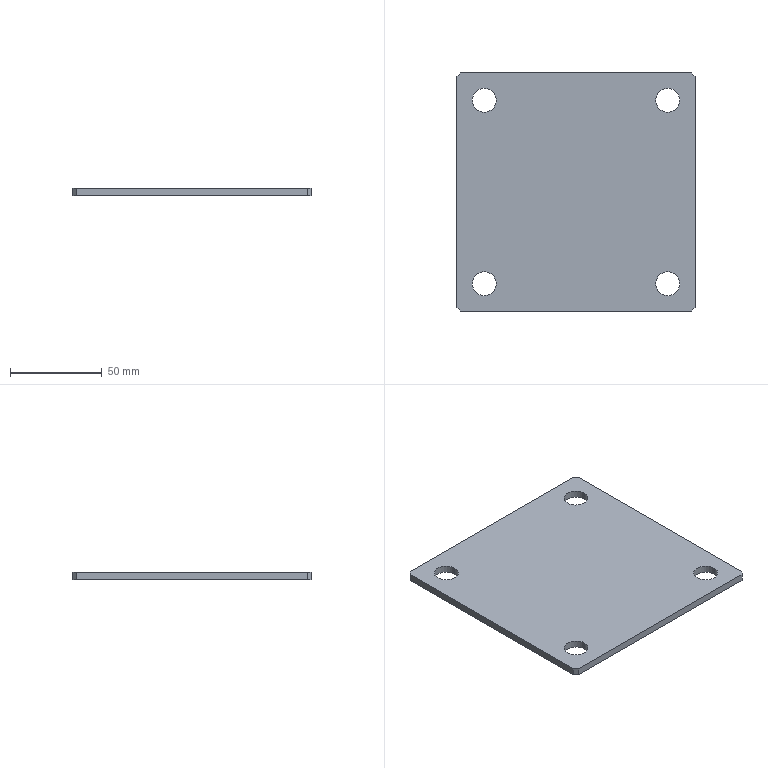Part | SolidWorks | features Chamfer 1, Extrusion 1, HoleWzd 1 | 1 solid | 18 faces | box 130 x 130 x 4 mm | volume 65444 mm3 | plane 10 | cylinder 8 | commonest cylinder face diameters 13 x8
STEP:
#1=CARTESIAN_POINT('',(-8.5,50.,4.));
#2=VERTEX_POINT('',#1);
#3=CARTESIAN_POINT('',(-21.5,50.,4.));
#4=VERTEX_POINT('',#3);
#5=CARTESIAN_POINT('',(-15.,50.,4.));
#6=DIRECTION('',(0.,0.,-1.));
#7=DIRECTION('',(-1.,0.,0.));
#8=AXIS2_PLACEMENT_3D('',#5,#6,#7);
#9=CIRCLE('',#8,6.5);
#10=EDGE_CURVE('',#2,#4,#9,.T.);
#11=ORIENTED_EDGE('',*,*,#10,.F.);
#12=CARTESIAN_POINT('',(-8.5,50.,0.));
#13=VERTEX_POINT('',#12);
#14=CARTESIAN_POINT('',(-8.5,50.,0.));
#15=DIRECTION('',(0.,0.,-1.));
#16=VECTOR('',#15,1000.);
#17=LINE('',#14,#16);
#18=EDGE_CURVE('',#2,#13,#17,.T.);
#19=ORIENTED_EDGE('',*,*,#18,.T.);
#20=CARTESIAN_POINT('',(-21.5,50.,0.));
#21=VERTEX_POINT('',#20);
#22=CARTESIAN_POINT('',(-15.,50.,0.));
#23=DIRECTION('',(0.,0.,-1.));
#24=DIRECTION('',(-1.,0.,0.));
#25=AXIS2_PLACEMENT_3D('',#22,#23,#24);
#26=CIRCLE('',#25,6.5);
#27=EDGE_CURVE('',#13,#21,#26,.T.);
#28=ORIENTED_EDGE('',*,*,#27,.T.);
#29=CARTESIAN_POINT('',(-21.5,50.,0.));
#30=DIRECTION('',(0.,0.,-1.));
#31=VECTOR('',#30,1000.);
#32=LINE('',#29,#31);
#33=EDGE_CURVE('',#4,#21,#32,.T.);
#34=ORIENTED_EDGE('',*,*,#33,.F.);
#35=EDGE_LOOP('',(#11,#19,#28,#34));
#36=FACE_OUTER_BOUND('',#35,.T.);
#37=CARTESIAN_POINT('',(-15.,50.,0.));
#38=DIRECTION('',(0.,0.,-1.));
#39=DIRECTION('',(-1.,0.,0.));
#40=AXIS2_PLACEMENT_3D('',#37,#38,#39);
#41=CYLINDRICAL_SURFACE('',#40,6.5);
#42=ADVANCED_FACE('',(#36),#41,.F.);
#43=CARTESIAN_POINT('',(-108.5,-50.,4.));
#44=VERTEX_POINT('',#43);
#45=CARTESIAN_POINT('',(-121.5,-50.,4.));
#46=VERTEX_POINT('',#45);
#47=CARTESIAN_POINT('',(-115.,-50.,4.));
#48=DIRECTION('',(0.,0.,-1.));
#49=DIRECTION('',(-1.,0.,0.));
#50=AXIS2_PLACEMENT_3D('',#47,#48,#49);
#51=CIRCLE('',#50,6.5);
#52=EDGE_CURVE('',#44,#46,#51,.T.);
#53=ORIENTED_EDGE('',*,*,#52,.F.);
#54=CARTESIAN_POINT('',(-108.5,-50.,0.));
#55=VERTEX_POINT('',#54);
#56=CARTESIAN_POINT('',(-108.5,-50.,0.));
#57=DIRECTION('',(0.,0.,-1.));
#58=VECTOR('',#57,1000.);
#59=LINE('',#56,#58);
#60=EDGE_CURVE('',#44,#55,#59,.T.);
#61=ORIENTED_EDGE('',*,*,#60,.T.);
#62=CARTESIAN_POINT('',(-121.5,-50.,0.));
#63=VERTEX_POINT('',#62);
#64=CARTESIAN_POINT('',(-115.,-50.,0.));
#65=DIRECTION('',(0.,0.,-1.));
#66=DIRECTION('',(-1.,0.,0.));
#67=AXIS2_PLACEMENT_3D('',#64,#65,#66);
#68=CIRCLE('',#67,6.5);
#69=EDGE_CURVE('',#55,#63,#68,.T.);
#70=ORIENTED_EDGE('',*,*,#69,.T.);
#71=CARTESIAN_POINT('',(-121.5,-50.,0.));
#72=DIRECTION('',(0.,0.,-1.));
#73=VECTOR('',#72,1000.);
#74=LINE('',#71,#73);
#75=EDGE_CURVE('',#46,#63,#74,.T.);
#76=ORIENTED_EDGE('',*,*,#75,.F.);
#77=EDGE_LOOP('',(#53,#61,#70,#76));
#78=FACE_OUTER_BOUND('',#77,.T.);
#79=CARTESIAN_POINT('',(-115.,-50.,0.));
#80=DIRECTION('',(0.,0.,-1.));
#81=DIRECTION('',(-1.,0.,0.));
#82=AXIS2_PLACEMENT_3D('',#79,#80,#81);
#83=CYLINDRICAL_SURFACE('',#82,6.5);
#84=ADVANCED_FACE('',(#78),#83,.F.);
#85=CARTESIAN_POINT('',(-108.5,50.,4.));
#86=VERTEX_POINT('',#85);
#87=CARTESIAN_POINT('',(-121.5,50.,4.));
#88=VERTEX_POINT('',#87);
#89=CARTESIAN_POINT('',(-115.,50.,4.));
#90=DIRECTION('',(0.,0.,-1.));
#91=DIRECTION('',(-1.,0.,0.));
#92=AXIS2_PLACEMENT_3D('',#89,#90,#91);
#93=CIRCLE('',#92,6.5);
#94=EDGE_CURVE('',#86,#88,#93,.T.);
#95=ORIENTED_EDGE('',*,*,#94,.F.);
#96=CARTESIAN_POINT('',(-108.5,50.,0.));
#97=VERTEX_POINT('',#96);
#98=CARTESIAN_POINT('',(-108.5,50.,0.));
#99=DIRECTION('',(0.,0.,-1.));
#100=VECTOR('',#99,1000.);
#101=LINE('',#98,#100);
#102=EDGE_CURVE('',#86,#97,#101,.T.);
#103=ORIENTED_EDGE('',*,*,#102,.T.);
#104=CARTESIAN_POINT('',(-121.5,50.,0.));
#105=VERTEX_POINT('',#104);
#106=CARTESIAN_POINT('',(-115.,50.,0.));
#107=DIRECTION('',(0.,0.,-1.));
#108=DIRECTION('',(-1.,0.,0.));
#109=AXIS2_PLACEMENT_3D('',#106,#107,#108);
#110=CIRCLE('',#109,6.5);
#111=EDGE_CURVE('',#97,#105,#110,.T.);
#112=ORIENTED_EDGE('',*,*,#111,.T.);
#113=CARTESIAN_POINT('',(-121.5,50.,0.));
#114=DIRECTION('',(0.,0.,-1.));
#115=VECTOR('',#114,1000.);
#116=LINE('',#113,#115);
#117=EDGE_CURVE('',#88,#105,#116,.T.);
#118=ORIENTED_EDGE('',*,*,#117,.F.);
#119=EDGE_LOOP('',(#95,#103,#112,#118));
#120=FACE_OUTER_BOUND('',#119,.T.);
#121=CARTESIAN_POINT('',(-115.,50.,0.));
#122=DIRECTION('',(0.,0.,-1.));
#123=DIRECTION('',(-1.,0.,0.));
#124=AXIS2_PLACEMENT_3D('',#121,#122,#123);
#125=CYLINDRICAL_SURFACE('',#124,6.5);
#126=ADVANCED_FACE('',(#120),#125,.F.);
#127=CARTESIAN_POINT('',(-8.5,-50.,4.));
#128=VERTEX_POINT('',#127);
#129=CARTESIAN_POINT('',(-21.5,-50.,4.));
#130=VERTEX_POINT('',#129);
#131=CARTESIAN_POINT('',(-15.,-50.,4.));
#132=DIRECTION('',(0.,0.,-1.));
#133=DIRECTION('',(-1.,0.,0.));
#134=AXIS2_PLACEMENT_3D('',#131,#132,#133);
#135=CIRCLE('',#134,6.5);
#136=EDGE_CURVE('',#128,#130,#135,.T.);
#137=ORIENTED_EDGE('',*,*,#136,.F.);
#138=CARTESIAN_POINT('',(-8.5,-50.,0.));
#139=VERTEX_POINT('',#138);
#140=CARTESIAN_POINT('',(-8.5,-50.,0.));
#141=DIRECTION('',(0.,0.,-1.));
#142=VECTOR('',#141,1000.);
#143=LINE('',#140,#142);
#144=EDGE_CURVE('',#128,#139,#143,.T.);
#145=ORIENTED_EDGE('',*,*,#144,.T.);
#146=CARTESIAN_POINT('',(-21.5,-50.,0.));
#147=VERTEX_POINT('',#146);
#148=CARTESIAN_POINT('',(-15.,-50.,0.));
#149=DIRECTION('',(0.,0.,-1.));
#150=DIRECTION('',(-1.,0.,0.));
#151=AXIS2_PLACEMENT_3D('',#148,#149,#150);
#152=CIRCLE('',#151,6.5);
#153=EDGE_CURVE('',#139,#147,#152,.T.);
#154=ORIENTED_EDGE('',*,*,#153,.T.);
#155=CARTESIAN_POINT('',(-21.5,-50.,0.));
#156=DIRECTION('',(0.,0.,-1.));
#157=VECTOR('',#156,1000.);
#158=LINE('',#155,#157);
#159=EDGE_CURVE('',#130,#147,#158,.T.);
#160=ORIENTED_EDGE('',*,*,#159,.F.);
#161=EDGE_LOOP('',(#137,#145,#154,#160));
#162=FACE_OUTER_BOUND('',#161,.T.);
#163=CARTESIAN_POINT('',(-15.,-50.,0.));
#164=DIRECTION('',(0.,0.,-1.));
#165=DIRECTION('',(-1.,0.,0.));
#166=AXIS2_PLACEMENT_3D('',#163,#164,#165);
#167=CYLINDRICAL_SURFACE('',#166,6.5);
#168=ADVANCED_FACE('',(#162),#167,.F.);
#169=CARTESIAN_POINT('',(0.,-63.,4.));
#170=VERTEX_POINT('',#169);
#171=CARTESIAN_POINT('',(0.,63.,4.));
#172=VERTEX_POINT('',#171);
#173=CARTESIAN_POINT('',(0.,65.,4.));
#174=DIRECTION('',(0.,1.,0.));
#175=VECTOR('',#174,1000.);
#176=LINE('',#173,#175);
#177=EDGE_CURVE('',#170,#172,#176,.T.);
#178=ORIENTED_EDGE('',*,*,#177,.F.);
#179=CARTESIAN_POINT('',(0.,-63.,0.));
#180=VERTEX_POINT('',#179);
#181=CARTESIAN_POINT('',(0.,-63.,4.));
#182=DIRECTION('',(0.,0.,-1.));
#183=VECTOR('',#182,1000.);
#184=LINE('',#181,#183);
#185=EDGE_CURVE('',#170,#180,#184,.T.);
#186=ORIENTED_EDGE('',*,*,#185,.T.);
#187=CARTESIAN_POINT('',(0.,63.,0.));
#188=VERTEX_POINT('',#187);
#189=CARTESIAN_POINT('',(0.,65.,0.));
#190=DIRECTION('',(0.,1.,0.));
#191=VECTOR('',#190,1000.);
#192=LINE('',#189,#191);
#193=EDGE_CURVE('',#180,#188,#192,.T.);
#194=ORIENTED_EDGE('',*,*,#193,.T.);
#195=CARTESIAN_POINT('',(0.,63.,4.));
#196=DIRECTION('',(0.,0.,1.));
#197=VECTOR('',#196,1000.);
#198=LINE('',#195,#197);
#199=EDGE_CURVE('',#188,#172,#198,.T.);
#200=ORIENTED_EDGE('',*,*,#199,.T.);
#201=EDGE_LOOP('',(#178,#186,#194,#200));
#202=FACE_OUTER_BOUND('',#201,.T.);
#203=CARTESIAN_POINT('',(0.,65.,4.));
#204=DIRECTION('',(-1.,0.,0.));
#205=DIRECTION('',(0.,-1.,0.));
#206=AXIS2_PLACEMENT_3D('',#203,#204,#205);
#207=PLANE('',#206);
#208=ADVANCED_FACE('',(#202),#207,.F.);
#209=CARTESIAN_POINT('',(-2.,65.,0.));
#210=VERTEX_POINT('',#209);
#211=CARTESIAN_POINT('',(-128.,65.,0.));
#212=VERTEX_POINT('',#211);
#213=CARTESIAN_POINT('',(0.,65.,0.));
#214=DIRECTION('',(-1.,0.,0.));
#215=VECTOR('',#214,1000.);
#216=LINE('',#213,#215);
#217=EDGE_CURVE('',#210,#212,#216,.T.);
#218=ORIENTED_EDGE('',*,*,#217,.T.);
#219=CARTESIAN_POINT('',(-128.,65.,4.));
#220=VERTEX_POINT('',#219);
#221=CARTESIAN_POINT('',(-128.,65.,4.));
#222=DIRECTION('',(0.,0.,1.));
#223=VECTOR('',#222,1000.);
#224=LINE('',#221,#223);
#225=EDGE_CURVE('',#212,#220,#224,.T.);
#226=ORIENTED_EDGE('',*,*,#225,.T.);
#227=CARTESIAN_POINT('',(-2.,65.,4.));
#228=VERTEX_POINT('',#227);
#229=CARTESIAN_POINT('',(0.,65.,4.));
#230=DIRECTION('',(-1.,0.,0.));
#231=VECTOR('',#230,1000.);
#232=LINE('',#229,#231);
#233=EDGE_CURVE('',#228,#220,#232,.T.);
#234=ORIENTED_EDGE('',*,*,#233,.F.);
#235=CARTESIAN_POINT('',(-2.,65.,4.));
#236=DIRECTION('',(0.,0.,-1.));
#237=VECTOR('',#236,1000.);
#238=LINE('',#235,#237);
#239=EDGE_CURVE('',#228,#210,#238,.T.);
#240=ORIENTED_EDGE('',*,*,#239,.T.);
#241=EDGE_LOOP('',(#218,#226,#234,#240));
#242=FACE_OUTER_BOUND('',#241,.T.);
#243=CARTESIAN_POINT('',(0.,65.,4.));
#244=DIRECTION('',(0.,-1.,0.));
#245=DIRECTION('',(0.,0.,-1.));
#246=AXIS2_PLACEMENT_3D('',#243,#244,#245);
#247=PLANE('',#246);
#248=ADVANCED_FACE('',(#242),#247,.F.);
#249=CARTESIAN_POINT('',(-130.,63.,4.));
#250=VERTEX_POINT('',#249);
#251=CARTESIAN_POINT('',(-130.,-63.,4.));
#252=VERTEX_POINT('',#251);
#253=CARTESIAN_POINT('',(-130.,65.,4.));
#254=DIRECTION('',(0.,-1.,0.));
#255=VECTOR('',#254,1000.);
#256=LINE('',#253,#255);
#257=EDGE_CURVE('',#250,#252,#256,.T.);
#258=ORIENTED_EDGE('',*,*,#257,.F.);
#259=CARTESIAN_POINT('',(-130.,63.,0.));
#260=VERTEX_POINT('',#259);
#261=CARTESIAN_POINT('',(-130.,63.,4.));
#262=DIRECTION('',(0.,0.,-1.));
#263=VECTOR('',#262,1000.);
#264=LINE('',#261,#263);
#265=EDGE_CURVE('',#250,#260,#264,.T.);
#266=ORIENTED_EDGE('',*,*,#265,.T.);
#267=CARTESIAN_POINT('',(-130.,-63.,0.));
#268=VERTEX_POINT('',#267);
#269=CARTESIAN_POINT('',(-130.,65.,0.));
#270=DIRECTION('',(0.,-1.,0.));
#271=VECTOR('',#270,1000.);
#272=LINE('',#269,#271);
#273=EDGE_CURVE('',#260,#268,#272,.T.);
#274=ORIENTED_EDGE('',*,*,#273,.T.);
#275=CARTESIAN_POINT('',(-130.,-63.,4.));
#276=DIRECTION('',(0.,0.,1.));
#277=VECTOR('',#276,1000.);
#278=LINE('',#275,#277);
#279=EDGE_CURVE('',#268,#252,#278,.T.);
#280=ORIENTED_EDGE('',*,*,#279,.T.);
#281=EDGE_LOOP('',(#258,#266,#274,#280));
#282=FACE_OUTER_BOUND('',#281,.T.);
#283=CARTESIAN_POINT('',(-130.,65.,4.));
#284=DIRECTION('',(1.,0.,0.));
#285=DIRECTION('',(0.,1.,0.));
#286=AXIS2_PLACEMENT_3D('',#283,#284,#285);
#287=PLANE('',#286);
#288=ADVANCED_FACE('',(#282),#287,.F.);
#289=CARTESIAN_POINT('',(-128.,-65.,4.));
#290=VERTEX_POINT('',#289);
#291=CARTESIAN_POINT('',(-2.,-65.,4.));
#292=VERTEX_POINT('',#291);
#293=CARTESIAN_POINT('',(0.,-65.,4.));
#294=DIRECTION('',(1.,0.,0.));
#295=VECTOR('',#294,1000.);
#296=LINE('',#293,#295);
#297=EDGE_CURVE('',#290,#292,#296,.T.);
#298=ORIENTED_EDGE('',*,*,#297,.F.);
#299=CARTESIAN_POINT('',(-128.,-65.,0.));
#300=VERTEX_POINT('',#299);
#301=CARTESIAN_POINT('',(-128.,-65.,4.));
#302=DIRECTION('',(0.,0.,-1.));
#303=VECTOR('',#302,1000.);
#304=LINE('',#301,#303);
#305=EDGE_CURVE('',#290,#300,#304,.T.);
#306=ORIENTED_EDGE('',*,*,#305,.T.);
#307=CARTESIAN_POINT('',(-2.,-65.,0.));
#308=VERTEX_POINT('',#307);
#309=CARTESIAN_POINT('',(0.,-65.,0.));
#310=DIRECTION('',(1.,0.,0.));
#311=VECTOR('',#310,1000.);
#312=LINE('',#309,#311);
#313=EDGE_CURVE('',#300,#308,#312,.T.);
#314=ORIENTED_EDGE('',*,*,#313,.T.);
#315=CARTESIAN_POINT('',(-2.,-65.,4.));
#316=DIRECTION('',(0.,0.,1.));
#317=VECTOR('',#316,1000.);
#318=LINE('',#315,#317);
#319=EDGE_CURVE('',#308,#292,#318,.T.);
#320=ORIENTED_EDGE('',*,*,#319,.T.);
#321=EDGE_LOOP('',(#298,#306,#314,#320));
#322=FACE_OUTER_BOUND('',#321,.T.);
#323=CARTESIAN_POINT('',(0.,-65.,4.));
#324=DIRECTION('',(0.,1.,0.));
#325=DIRECTION('',(-1.,0.,0.));
#326=AXIS2_PLACEMENT_3D('',#323,#324,#325);
#327=PLANE('',#326);
#328=ADVANCED_FACE('',(#322),#327,.F.);
#329=CARTESIAN_POINT('',(-15.,50.,4.));
#330=DIRECTION('',(0.,0.,-1.));
#331=DIRECTION('',(-1.,0.,0.));
#332=AXIS2_PLACEMENT_3D('',#329,#330,#331);
#333=CIRCLE('',#332,6.5);
#334=EDGE_CURVE('',#4,#2,#333,.T.);
#335=ORIENTED_EDGE('',*,*,#334,.T.);
#336=ORIENTED_EDGE('',*,*,#10,.T.);
#337=EDGE_LOOP('',(#335,#336));
#338=FACE_BOUND('',#337,.T.);
#339=CARTESIAN_POINT('',(-115.,-50.,4.));
#340=DIRECTION('',(0.,0.,-1.));
#341=DIRECTION('',(-1.,0.,0.));
#342=AXIS2_PLACEMENT_3D('',#339,#340,#341);
#343=CIRCLE('',#342,6.5);
#344=EDGE_CURVE('',#46,#44,#343,.T.);
#345=ORIENTED_EDGE('',*,*,#344,.T.);
#346=ORIENTED_EDGE('',*,*,#52,.T.);
#347=EDGE_LOOP('',(#345,#346));
#348=FACE_BOUND('',#347,.T.);
#349=CARTESIAN_POINT('',(-115.,50.,4.));
#350=DIRECTION('',(0.,0.,-1.));
#351=DIRECTION('',(-1.,0.,0.));
#352=AXIS2_PLACEMENT_3D('',#349,#350,#351);
#353=CIRCLE('',#352,6.5);
#354=EDGE_CURVE('',#88,#86,#353,.T.);
#355=ORIENTED_EDGE('',*,*,#354,.T.);
#356=ORIENTED_EDGE('',*,*,#94,.T.);
#357=EDGE_LOOP('',(#355,#356));
#358=FACE_BOUND('',#357,.T.);
#359=CARTESIAN_POINT('',(-15.,-50.,4.));
#360=DIRECTION('',(0.,0.,-1.));
#361=DIRECTION('',(-1.,0.,0.));
#362=AXIS2_PLACEMENT_3D('',#359,#360,#361);
#363=CIRCLE('',#362,6.5);
#364=EDGE_CURVE('',#130,#128,#363,.T.);
#365=ORIENTED_EDGE('',*,*,#364,.T.);
#366=ORIENTED_EDGE('',*,*,#136,.T.);
#367=EDGE_LOOP('',(#365,#366));
#368=FACE_BOUND('',#367,.T.);
#369=ORIENTED_EDGE('',*,*,#233,.T.);
#370=CARTESIAN_POINT('',(-130.,63.,4.));
#371=DIRECTION('',(-0.7071,-0.7071,0.));
#372=VECTOR('',#371,1000.);
#373=LINE('',#370,#372);
#374=EDGE_CURVE('',#220,#250,#373,.T.);
#375=ORIENTED_EDGE('',*,*,#374,.T.);
#376=ORIENTED_EDGE('',*,*,#257,.T.);
#377=CARTESIAN_POINT('',(-128.,-65.,4.));
#378=DIRECTION('',(0.7071,-0.7071,0.));
#379=VECTOR('',#378,1000.);
#380=LINE('',#377,#379);
#381=EDGE_CURVE('',#252,#290,#380,.T.);
#382=ORIENTED_EDGE('',*,*,#381,.T.);
#383=ORIENTED_EDGE('',*,*,#297,.T.);
#384=CARTESIAN_POINT('',(0.,-63.,4.));
#385=DIRECTION('',(0.7071,0.7071,0.));
#386=VECTOR('',#385,1000.);
#387=LINE('',#384,#386);
#388=EDGE_CURVE('',#292,#170,#387,.T.);
#389=ORIENTED_EDGE('',*,*,#388,.T.);
#390=ORIENTED_EDGE('',*,*,#177,.T.);
#391=CARTESIAN_POINT('',(-2.,65.,4.));
#392=DIRECTION('',(-0.7071,0.7071,0.));
#393=VECTOR('',#392,1000.);
#394=LINE('',#391,#393);
#395=EDGE_CURVE('',#172,#228,#394,.T.);
#396=ORIENTED_EDGE('',*,*,#395,.T.);
#397=EDGE_LOOP('',(#369,#375,#376,#382,#383,#389,#390,#396));
#398=FACE_OUTER_BOUND('',#397,.T.);
#399=CARTESIAN_POINT('',(0.,0.,4.));
#400=DIRECTION('',(0.,0.,-1.));
#401=DIRECTION('',(-1.,0.,0.));
#402=AXIS2_PLACEMENT_3D('',#399,#400,#401);
#403=PLANE('',#402);
#404=ADVANCED_FACE('',(#338,#348,#358,#368,#398),#403,.F.);
#405=CARTESIAN_POINT('',(-15.,50.,0.));
#406=DIRECTION('',(0.,0.,-1.));
#407=DIRECTION('',(-1.,0.,0.));
#408=AXIS2_PLACEMENT_3D('',#405,#406,#407);
#409=CIRCLE('',#408,6.5);
#410=EDGE_CURVE('',#21,#13,#409,.T.);
#411=ORIENTED_EDGE('',*,*,#410,.F.);
#412=ORIENTED_EDGE('',*,*,#27,.F.);
#413=EDGE_LOOP('',(#411,#412));
#414=FACE_BOUND('',#413,.T.);
#415=CARTESIAN_POINT('',(-115.,-50.,0.));
#416=DIRECTION('',(0.,0.,-1.));
#417=DIRECTION('',(-1.,0.,0.));
#418=AXIS2_PLACEMENT_3D('',#415,#416,#417);
#419=CIRCLE('',#418,6.5);
#420=EDGE_CURVE('',#63,#55,#419,.T.);
#421=ORIENTED_EDGE('',*,*,#420,.F.);
#422=ORIENTED_EDGE('',*,*,#69,.F.);
#423=EDGE_LOOP('',(#421,#422));
#424=FACE_BOUND('',#423,.T.);
#425=CARTESIAN_POINT('',(-115.,50.,0.));
#426=DIRECTION('',(0.,0.,-1.));
#427=DIRECTION('',(-1.,0.,0.));
#428=AXIS2_PLACEMENT_3D('',#425,#426,#427);
#429=CIRCLE('',#428,6.5);
#430=EDGE_CURVE('',#105,#97,#429,.T.);
#431=ORIENTED_EDGE('',*,*,#430,.F.);
#432=ORIENTED_EDGE('',*,*,#111,.F.);
#433=EDGE_LOOP('',(#431,#432));
#434=FACE_BOUND('',#433,.T.);
#435=CARTESIAN_POINT('',(-15.,-50.,0.));
#436=DIRECTION('',(0.,0.,-1.));
#437=DIRECTION('',(-1.,0.,0.));
#438=AXIS2_PLACEMENT_3D('',#435,#436,#437);
#439=CIRCLE('',#438,6.5);
#440=EDGE_CURVE('',#147,#139,#439,.T.);
#441=ORIENTED_EDGE('',*,*,#440,.F.);
#442=ORIENTED_EDGE('',*,*,#153,.F.);
#443=EDGE_LOOP('',(#441,#442));
#444=FACE_BOUND('',#443,.T.);
#445=ORIENTED_EDGE('',*,*,#273,.F.);
#446=CARTESIAN_POINT('',(-96.5,96.5,0.));
#447=DIRECTION('',(0.7071,0.7071,0.));
#448=VECTOR('',#447,1000.);
#449=LINE('',#446,#448);
#450=EDGE_CURVE('',#260,#212,#449,.T.);
#451=ORIENTED_EDGE('',*,*,#450,.T.);
#452=ORIENTED_EDGE('',*,*,#217,.F.);
#453=CARTESIAN_POINT('',(31.5,31.5,0.));
#454=DIRECTION('',(0.7071,-0.7071,0.));
#455=VECTOR('',#454,1000.);
#456=LINE('',#453,#455);
#457=EDGE_CURVE('',#210,#188,#456,.T.);
#458=ORIENTED_EDGE('',*,*,#457,.T.);
#459=ORIENTED_EDGE('',*,*,#193,.F.);
#460=CARTESIAN_POINT('',(31.5,-31.5,0.));
#461=DIRECTION('',(-0.7071,-0.7071,0.));
#462=VECTOR('',#461,1000.);
#463=LINE('',#460,#462);
#464=EDGE_CURVE('',#180,#308,#463,.T.);
#465=ORIENTED_EDGE('',*,*,#464,.T.);
#466=ORIENTED_EDGE('',*,*,#313,.F.);
#467=CARTESIAN_POINT('',(-96.5,-96.5,0.));
#468=DIRECTION('',(-0.7071,0.7071,0.));
#469=VECTOR('',#468,1000.);
#470=LINE('',#467,#469);
#471=EDGE_CURVE('',#300,#268,#470,.T.);
#472=ORIENTED_EDGE('',*,*,#471,.T.);
#473=EDGE_LOOP('',(#445,#451,#452,#458,#459,#465,#466,#472));
#474=FACE_OUTER_BOUND('',#473,.T.);
#475=CARTESIAN_POINT('',(0.,0.,0.));
#476=DIRECTION('',(0.,0.,-1.));
#477=DIRECTION('',(-1.,0.,0.));
#478=AXIS2_PLACEMENT_3D('',#475,#476,#477);
#479=PLANE('',#478);
#480=ADVANCED_FACE('',(#414,#424,#434,#444,#474),#479,.T.);
#481=ORIENTED_EDGE('',*,*,#374,.F.);
#482=ORIENTED_EDGE('',*,*,#225,.F.);
#483=ORIENTED_EDGE('',*,*,#450,.F.);
#484=ORIENTED_EDGE('',*,*,#265,.F.);
#485=EDGE_LOOP('',(#481,#482,#483,#484));
#486=FACE_OUTER_BOUND('',#485,.T.);
#487=CARTESIAN_POINT('',(-130.,63.,4.));
#488=DIRECTION('',(0.7071,-0.7071,0.));
#489=DIRECTION('',(0.,0.,-1.));
#490=AXIS2_PLACEMENT_3D('',#487,#488,#489);
#491=PLANE('',#490);
#492=ADVANCED_FACE('',(#486),#491,.F.);
#493=ORIENTED_EDGE('',*,*,#381,.F.);
#494=ORIENTED_EDGE('',*,*,#279,.F.);
#495=ORIENTED_EDGE('',*,*,#471,.F.);
#496=ORIENTED_EDGE('',*,*,#305,.F.);
#497=EDGE_LOOP('',(#493,#494,#495,#496));
#498=FACE_OUTER_BOUND('',#497,.T.);
#499=CARTESIAN_POINT('',(-128.,-65.,4.));
#500=DIRECTION('',(0.7071,0.7071,0.));
#501=DIRECTION('',(0.,0.,-1.));
#502=AXIS2_PLACEMENT_3D('',#499,#500,#501);
#503=PLANE('',#502);
#504=ADVANCED_FACE('',(#498),#503,.F.);
#505=ORIENTED_EDGE('',*,*,#388,.F.);
#506=ORIENTED_EDGE('',*,*,#319,.F.);
#507=ORIENTED_EDGE('',*,*,#464,.F.);
#508=ORIENTED_EDGE('',*,*,#185,.F.);
#509=EDGE_LOOP('',(#505,#506,#507,#508));
#510=FACE_OUTER_BOUND('',#509,.T.);
#511=CARTESIAN_POINT('',(0.,-63.,4.));
#512=DIRECTION('',(-0.7071,0.7071,0.));
#513=DIRECTION('',(0.,0.,-1.));
#514=AXIS2_PLACEMENT_3D('',#511,#512,#513);
#515=PLANE('',#514);
#516=ADVANCED_FACE('',(#510),#515,.F.);
#517=ORIENTED_EDGE('',*,*,#395,.F.);
#518=ORIENTED_EDGE('',*,*,#199,.F.);
#519=ORIENTED_EDGE('',*,*,#457,.F.);
#520=ORIENTED_EDGE('',*,*,#239,.F.);
#521=EDGE_LOOP('',(#517,#518,#519,#520));
#522=FACE_OUTER_BOUND('',#521,.T.);
#523=CARTESIAN_POINT('',(-2.,65.,4.));
#524=DIRECTION('',(-0.7071,-0.7071,0.));
#525=DIRECTION('',(0.,0.,-1.));
#526=AXIS2_PLACEMENT_3D('',#523,#524,#525);
#527=PLANE('',#526);
#528=ADVANCED_FACE('',(#522),#527,.F.);
#529=ORIENTED_EDGE('',*,*,#144,.F.);
#530=ORIENTED_EDGE('',*,*,#364,.F.);
#531=ORIENTED_EDGE('',*,*,#159,.T.);
#532=ORIENTED_EDGE('',*,*,#440,.T.);
#533=EDGE_LOOP('',(#529,#530,#531,#532));
#534=FACE_OUTER_BOUND('',#533,.T.);
#535=CARTESIAN_POINT('',(-15.,-50.,0.));
#536=DIRECTION('',(0.,0.,-1.));
#537=DIRECTION('',(-1.,0.,0.));
#538=AXIS2_PLACEMENT_3D('',#535,#536,#537);
#539=CYLINDRICAL_SURFACE('',#538,6.5);
#540=ADVANCED_FACE('',(#534),#539,.F.);
#541=ORIENTED_EDGE('',*,*,#102,.F.);
#542=ORIENTED_EDGE('',*,*,#354,.F.);
#543=ORIENTED_EDGE('',*,*,#117,.T.);
#544=ORIENTED_EDGE('',*,*,#430,.T.);
#545=EDGE_LOOP('',(#541,#542,#543,#544));
#546=FACE_OUTER_BOUND('',#545,.T.);
#547=CARTESIAN_POINT('',(-115.,50.,0.));
#548=DIRECTION('',(0.,0.,-1.));
#549=DIRECTION('',(-1.,0.,0.));
#550=AXIS2_PLACEMENT_3D('',#547,#548,#549);
#551=CYLINDRICAL_SURFACE('',#550,6.5);
#552=ADVANCED_FACE('',(#546),#551,.F.);
#553=ORIENTED_EDGE('',*,*,#60,.F.);
#554=ORIENTED_EDGE('',*,*,#344,.F.);
#555=ORIENTED_EDGE('',*,*,#75,.T.);
#556=ORIENTED_EDGE('',*,*,#420,.T.);
#557=EDGE_LOOP('',(#553,#554,#555,#556));
#558=FACE_OUTER_BOUND('',#557,.T.);
#559=CARTESIAN_POINT('',(-115.,-50.,0.));
#560=DIRECTION('',(0.,0.,-1.));
#561=DIRECTION('',(-1.,0.,0.));
#562=AXIS2_PLACEMENT_3D('',#559,#560,#561);
#563=CYLINDRICAL_SURFACE('',#562,6.5);
#564=ADVANCED_FACE('',(#558),#563,.F.);
#565=ORIENTED_EDGE('',*,*,#18,.F.);
#566=ORIENTED_EDGE('',*,*,#334,.F.);
#567=ORIENTED_EDGE('',*,*,#33,.T.);
#568=ORIENTED_EDGE('',*,*,#410,.T.);
#569=EDGE_LOOP('',(#565,#566,#567,#568));
#570=FACE_OUTER_BOUND('',#569,.T.);
#571=CARTESIAN_POINT('',(-15.,50.,0.));
#572=DIRECTION('',(0.,0.,-1.));
#573=DIRECTION('',(-1.,0.,0.));
#574=AXIS2_PLACEMENT_3D('',#571,#572,#573);
#575=CYLINDRICAL_SURFACE('',#574,6.5);
#576=ADVANCED_FACE('',(#570),#575,.F.);
#577=CLOSED_SHELL('',(#42,#84,#126,#168,#208,#248,#288,#328,#404,#480,#492,#504,#516,#528,#540,#552,#564,#576));
#578=MANIFOLD_SOLID_BREP('',#577);
#579=CARTESIAN_POINT('',(0.,0.,0.));
#580=DIRECTION('',(0.,0.,1.));
#581=DIRECTION('',(1.,0.,0.));
#582=AXIS2_PLACEMENT_3D('',#579,#580,#581);
#583=(LENGTH_UNIT()NAMED_UNIT(*)SI_UNIT(.MILLI.,.METRE.));
#584=UNCERTAINTY_MEASURE_WITH_UNIT(LENGTH_MEASURE(0.00001),#583,'','');
#585=(NAMED_UNIT(*)PLANE_ANGLE_UNIT()SI_UNIT($,.RADIAN.));
#586=(NAMED_UNIT(*)SI_UNIT($,.STERADIAN.)SOLID_ANGLE_UNIT());
#587=(GEOMETRIC_REPRESENTATION_CONTEXT(3)GLOBAL_UNCERTAINTY_ASSIGNED_CONTEXT((#584))GLOBAL_UNIT_ASSIGNED_CONTEXT((#583,#585,#586))REPRESENTATION_CONTEXT('',''));
#588=ADVANCED_BREP_SHAPE_REPRESENTATION('',(#578,#582),#587);